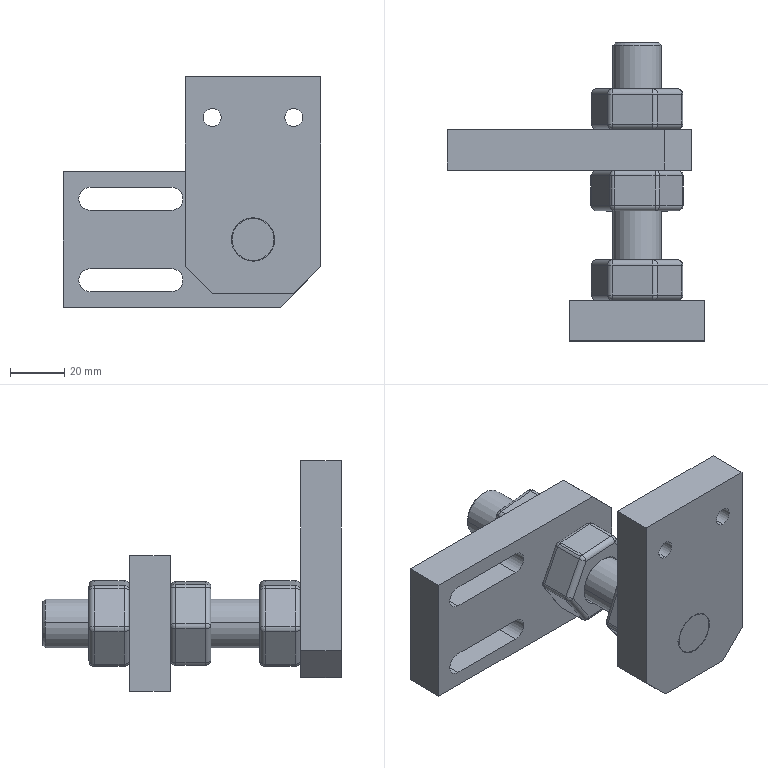Part | SolidWorks | 6 solids | 217 faces | box 95 x 110 x 85 mm | volume 155780 mm3 | cylinder 123 | plane 51 | sphere 36 | cone 4 | spline 3 | commonest cylinder face diameters 4 x57 18 x50 6.6 x4 8.4 x4 11 x4 15.5 x2